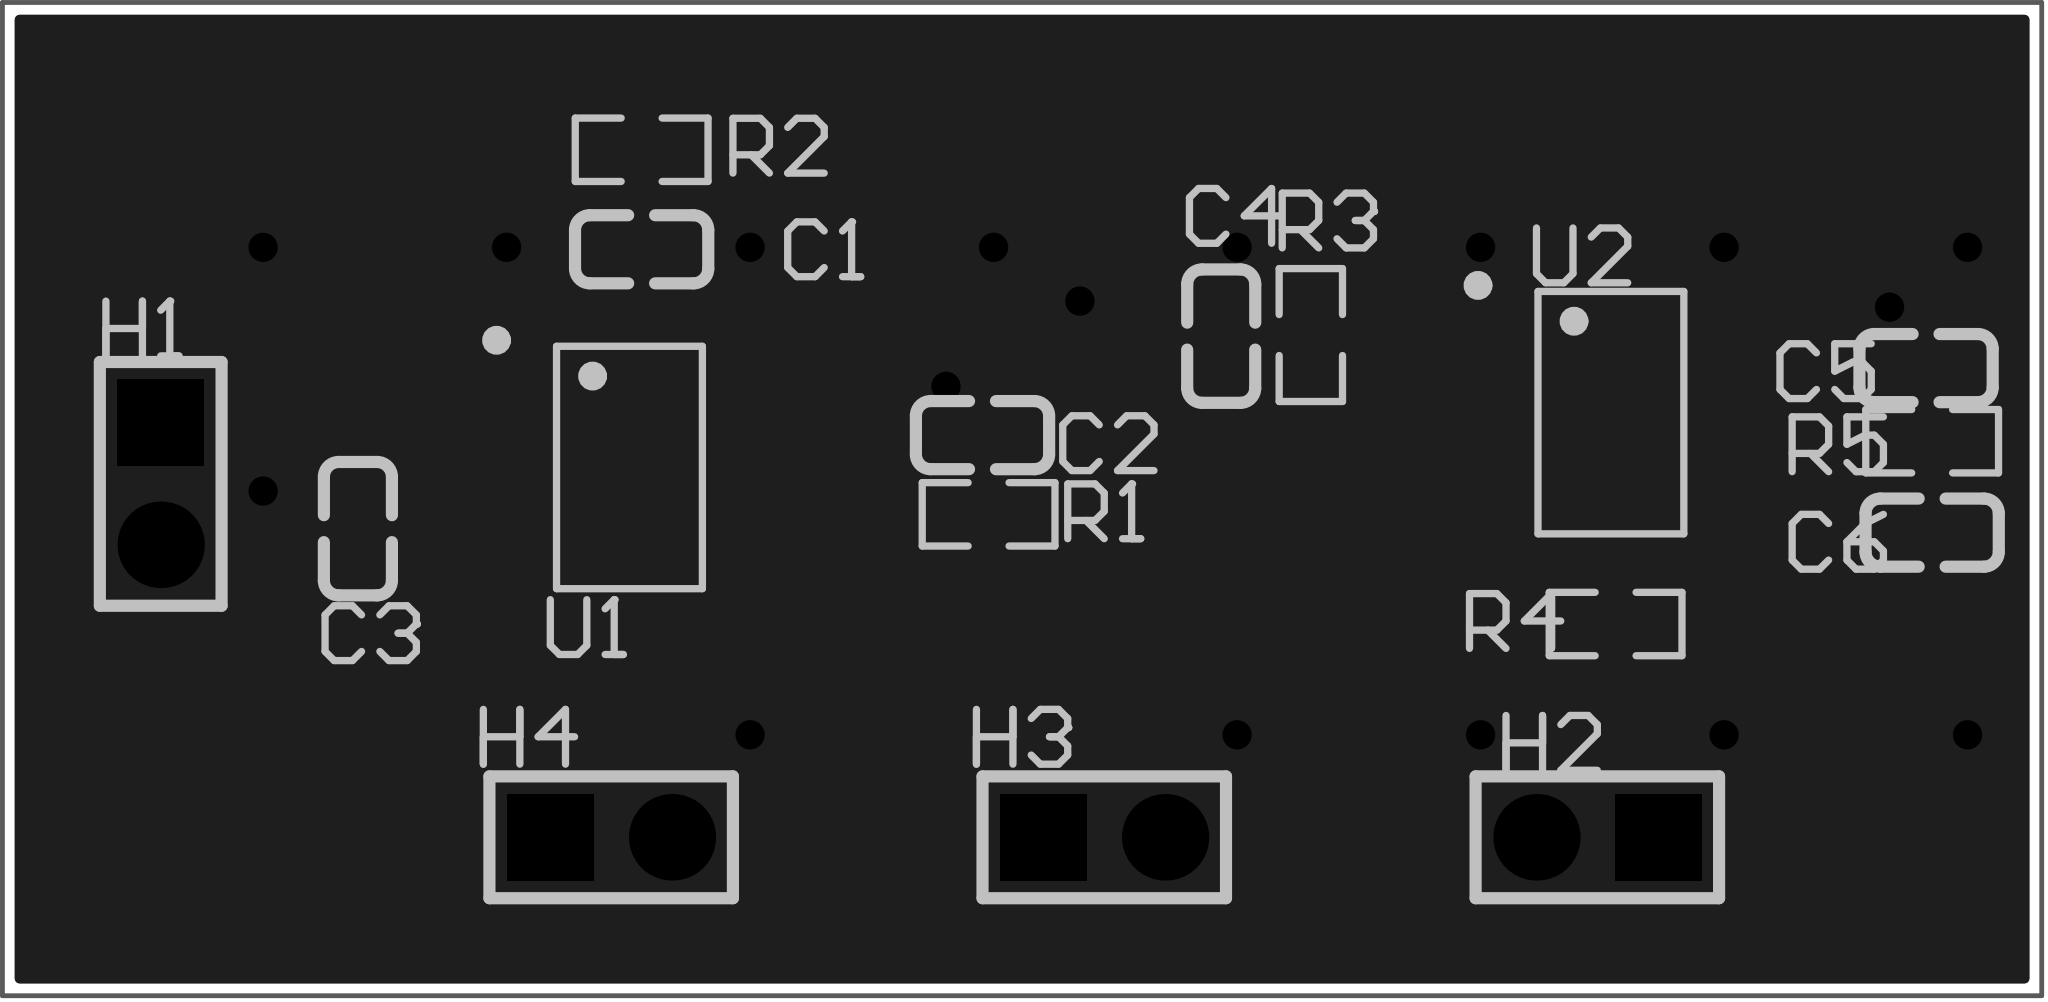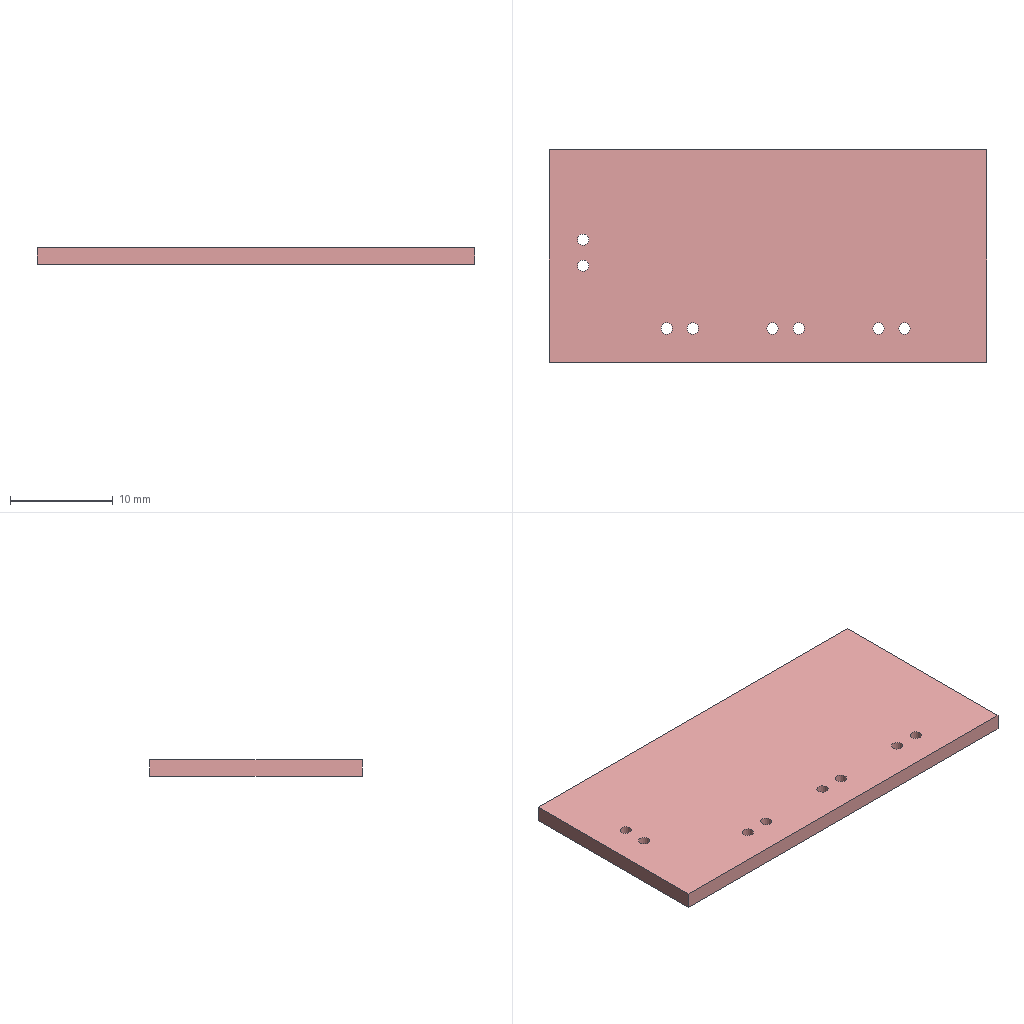Circuit board layout | Altium Designer | box 42.5 x 20.7 x 1.6 mm
Layer stack:
# Altium Designer layer stack of  (unit mm; dielectric type: 0 none, 1 core, 2 prepreg, 3 surface material)
index,name,kind,layer,copper_thickness_mm,dielectric_type,dielectric_thickness_mm,dielectric_material,dielectric_constant
0,Top Paste Mask Layer,other,,,,,,
1,Top Silkscreen Layer,other,,,,,,
2,Top Solder Mask Layer,dielectric,,,3,0.01,,3.3
3,Top Layer,copper,Top Layer,0.035,,,,
4,Dielectric1,dielectric,,,3,1.51,FR4,4.5
5,Bottom Layer,copper,Bottom Layer,0.035,,,,
6,Bottom Solder Mask Layer,dielectric,,,3,0.01,,3.3
7,Bottom Silkscreen Layer,other,,,,,,
8,Bottom Paste Mask Layer,other,,,,,,
# drill layer pairs: low layer,high layer
drill_pair,Top Layer,Bottom Layer
Part placement:
Designator,Comment,Layer,Footprint,Center-X(mm),Center-Y(mm),Rotation
C1,10nF,TopLayer,C0603,92.838,97.091,0
C2,100nF,TopLayer,C0603,99.949,93.218,180
C3,100nF,TopLayer,C0603,86.918,91.268,90
C4,100nF,TopLayer,C0603,104.929,95.281,90
C5,100nF,TopLayer,C0603,119.634,94.615,180
C6,100nF,TopLayer,C0603,119.761,91.186,180
H1,,TopLayer,HDR-TH_2P-P2.54-V-M-1,82.804,92.202,270
H2,,TopLayer,HDR-TH_2P-P2.54-V-M-1,112.776,84.836,180
H3,,TopLayer,HDR-TH_2P-P2.54-V-M-1,102.489,84.836,0
H4,,TopLayer,HDR-TH_2P-P2.54-V-M-1,92.202,84.836,0
R1,10K,TopLayer,R0603,100.076,91.567,0
R2,1. 1MEG,TopLayer,R0603,92.838,99.165,0
R3,8.2K,TopLayer,R0603,106.799,95.304,270
R4,120K,TopLayer,R0603,113.157,89.281,0
R5,5.1K,TopLayer,R0603,119.761,93.091,0
U1,OPA445AUG4,TopLayer,SOIC-8_L4.9-W3.9-P1.27-LS6.0-BL,92.584,92.544,270
U2,OPA445AUG4,TopLayer,SOIC-8_L4.9-W3.9-P1.27-LS6.0-BL,113.059,93.687,270
Pad and via stacks:
# Altium Designer via and pad stacks of  (unit mm). Each distinct definition once, with the count of objects using it.
# via: kind,start_layer,end_layer,hole_mm,diameter_mm,mode(0 simple;1 top-mid-bottom;2 full stack),diameter_per_layer,count,example_net
# pad: kind,layer,hole_mm,hole_type(0 round;1 square;2 slot),plating,top_size,top_shape(1 round;2 rect;3 octagon;9 rounded rect),mid_size,bottom_size,mode,footprint,size_per_layer,count,example
pad,Top Layer,0,0,plated,0.8x0.9,2,0.8x0.9,0.8x0.9,0,C0603,,12,C1.2
pad,Top Layer,0,0,plated,0.8065x0.864,2,0.8065x0.864,0.8065x0.864,0,R0603,,10,R1.2
pad,Top Layer,0,0,plated,0.588x2.045,1,0.588x2.045,0.588x2.045,0,SOIC-8_L4.9-W3.9-P1.27-LS6.0-BL,,16,U1.5
pad,Multi-Layer,1.1,0,plated,1.8x1.8,1,1.8x1.8,1.8x1.8,0,HDR-TH_2P-P2.54-V-M-1,,4,H1.2
pad,Multi-Layer,1.1,0,plated,1.8x1.8,2,1.8x1.8,1.8x1.8,0,HDR-TH_2P-P2.54-V-M-1,,4,H1.1
via,Top Layer,Bottom Layer,0.3048,0.61,0,,17,1V
Copper pours:
name,layer,net,type(0 solid;1 hatched;2 none)
Top Layer-GND,Top Layer,GND,0
Bottom Layer-GND,Bottom Layer,GND,0
Design rules, without the lines most boards share:
# Altium Designer design rules of  (exported by Altium Designer, unit mm)
# columns: name | kind | enabled | priority | scope1 | scope2 | descriptor | typed fields (field=value)
creepage | 65 | enabled | 1 | All | All | Creepage Distance Constraint =(0mil) (All),(All) |